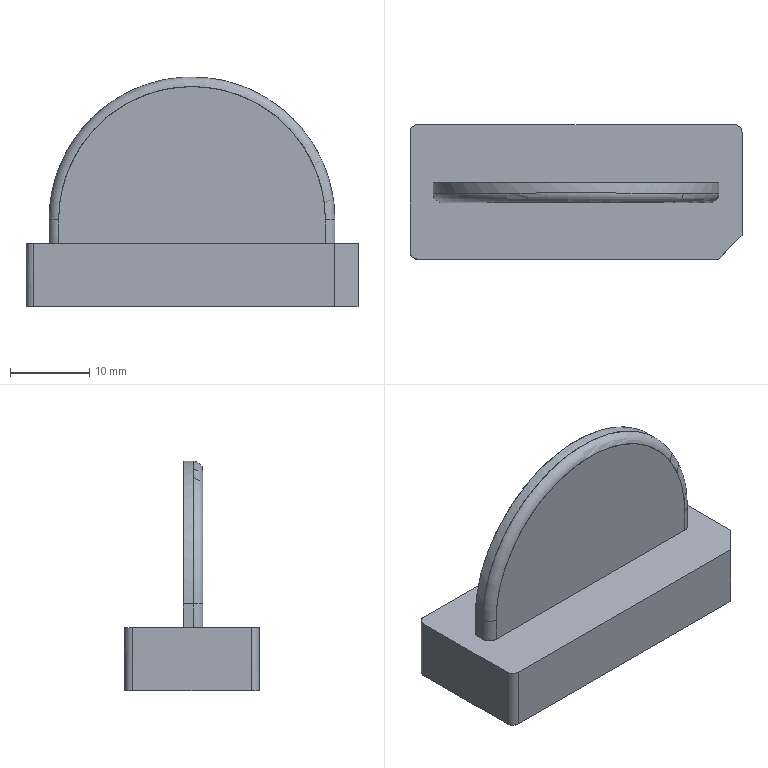NC program | PowerMill | posted with a generic post | part box 42 x 17 x 29.081 mm
Lines 14349 to 15047 of 145628:
N14446 M6
N14447 S18000 M03
N14448 G00 G90 X0.0 Y0.0
N14449 G43 Z10.798 H7
N14450
N14451 G05 P10000 R8
N14452 X19.2751 Y-2.1794
N14453 Z-19.2241
N14454 G01 Z-20.4241 F1200.0
N14455 X19.275 Y-2.1795 Z-20.2759 F2000.0
N14456 X19.2748 Y-2.1796 Z-20.2573
N14457 X19.2725 Y-2.1819 Z-20.1811
N14458 X19.2673 Y-2.1872 Z-20.0904
N14459 X19.2619 Y-2.1926 Z-20.0169
N14460 X19.2569 Y-2.1976 Z-19.9571
N14461 X19.2492 Y-2.2053 Z-19.8956
N14462 X19.2381 Y-2.2163 Z-19.8291
N14463 X19.2231 Y-2.2314 Z-19.7547
N14464 X19.2025 Y-2.252 Z-19.6656
N14465 X19.1985 Y-2.256 Z-19.6511
N14466 X19.1938 Y-2.2606 Z-19.637
N14467 X19.1865 Y-2.268 Z-19.6166
N14468 X19.1776 Y-2.2769 Z-19.5934
N14469 X19.1714 Y-2.2831 Z-19.5786
N14470 X19.1653 Y-2.2891 Z-19.5656
N14471 X19.1292 Y-2.3253 Z-19.5125
N14472 X19.0625 Y-2.392 Z-19.4813
N14473 X19.0133 Y-2.4412 Z-19.5198
N14474 X18.9993 Y-2.4552 Z-19.5402
N14475 X18.9861 Y-2.4683 Z-19.5629
N14476 X18.9759 Y-2.4786 Z-19.586
N14477 X18.9669 Y-2.4875 Z-19.6121
N14478 X18.959 Y-2.4955 Z-19.639
N14479 X18.9531 Y-2.5013 Z-19.6603
N14480 X18.9478 Y-2.5067 Z-19.6819
N14481 X18.9427 Y-2.5118 Z-19.7036
N14482 X18.9354 Y-2.5191 Z-19.7361
N14483 X18.9308 Y-2.5237 Z-19.758
N14484 X18.9266 Y-2.5279 Z-19.78
N14485 X18.9224 Y-2.5321 Z-19.8055
N14486 X18.9129 Y-2.5416 Z-19.8656
N14487 X18.9047 Y-2.5498 Z-19.9261
N14488 X18.8988 Y-2.5557 Z-19.9872
N14489 X18.8944 Y-2.5601 Z-20.0485
N14490 X18.8904 Y-2.5641 Z-20.1099
N14491 Z-20.1215
N14492 X18.8897 Y-2.5647 Z-20.2091
N14493 X18.8875 Y-2.567 Z-20.2763
N14494 X18.8874 Y-2.5671 Z-20.4235
N14495 X18.8013 Y-2.6369 Z-20.3989
N14496 X18.7127 Y-2.7036 Z-20.3742
N14497 X18.6217 Y-2.7671 Z-20.3496
N14498 X18.6066 Y-2.7772 Z-20.3456
N14499 Z-20.268
N14500 X18.6083 Y-2.7755 Z-20.1987
N14501 X18.6085 Y-2.7753 Z-20.1449
N14502 X18.6109 Y-2.7729 Z-20.0062
N14503 X18.6161 Y-2.7677 Z-19.8643
N14504 X18.6242 Y-2.7595 Z-19.7189
N14505 X18.6329 Y-2.7509 Z-19.6004
N14506 X18.6409 Y-2.7429 Z-19.5043
N14507 X18.65 Y-2.7337 Z-19.4084
N14508 X18.6613 Y-2.7224 Z-19.3129
N14509 X18.675 Y-2.7088 Z-19.2181
N14510 X18.69 Y-2.6937 Z-19.1236
N14511 X18.7028 Y-2.681 Z-19.0474
N14512 X18.7181 Y-2.6657 Z-18.9706
N14513 X18.7367 Y-2.647 Z-18.8916
N14514 X18.7587 Y-2.6251 Z-18.8107
N14515 X18.7831 Y-2.6007 Z-18.731
N14516 X18.7923 Y-2.5915 Z-18.7055
N14517 X18.8023 Y-2.5814 Z-18.6807
N14518 X18.817 Y-2.5668 Z-18.6469
N14519 X18.8281 Y-2.5557 Z-18.623
N14520 X18.8396 Y-2.5441 Z-18.5995
N14521 X18.852 Y-2.5318 Z-18.5768
N14522 X18.8729 Y-2.5109 Z-18.544
N14523 X18.8922 Y-2.4916 Z-18.5182
N14524 X18.911 Y-2.4728 Z-18.4977
N14525 X18.9297 Y-2.4541 Z-18.4817
N14526 X18.9473 Y-2.4365 Z-18.4705
N14527 X19.013 Y-2.3708 Z-18.4544
N14528 X19.088 Y-2.2957 Z-18.4839
N14529 X19.1086 Y-2.2752 Z-18.5007
N14530 X19.1295 Y-2.2543 Z-18.5222
N14531 X19.1514 Y-2.2324 Z-18.5494
N14532 X19.1702 Y-2.2135 Z-18.576
N14533 X19.1904 Y-2.1934 Z-18.6077
N14534 X19.2089 Y-2.1749 Z-18.6413
N14535 X19.2257 Y-2.158 Z-18.6767
N14536 X19.2483 Y-2.1355 Z-18.7258
N14537 X19.263 Y-2.1207 Z-18.7606
N14538 X19.2746 Y-2.1091 Z-18.7912
N14539 X19.2857 Y-2.0981 Z-18.8222
N14540 X19.2964 Y-2.0873 Z-18.8534
N14541 X19.3067 Y-2.0771 Z-18.885
N14542 X19.3277 Y-2.0561 Z-18.9543
N14543 X19.3469 Y-2.0369 Z-19.0247
N14544 X19.3642 Y-2.0196 Z-19.0963
N14545 X19.3796 Y-2.0041 Z-19.1685
N14546 X19.3937 Y-1.99 Z-19.2414
N14547 X19.4069 Y-1.9768 Z-19.3145
N14548 X19.4192 Y-1.9646 Z-19.3879
N14549 X19.4334 Y-1.9504 Z-19.4875
N14550 X19.447 Y-1.9368 Z-19.6012
N14551 X19.457 Y-1.9268 Z-19.6985
N14552 X19.4641 Y-1.9197 Z-19.7821
N14553 X19.4698 Y-1.914 Z-19.8659
N14554 X19.4745 Y-1.9093 Z-19.9499
N14555 X19.4783 Y-1.9055 Z-20.0339
N14556 X19.4809 Y-1.9029 Z-20.118
N14557 X19.4838 Y-1.9 Z-20.2678
N14558 X19.4839 Y-1.8999 Z-20.2719
N14559 Z-20.4005
N14560 X19.5967 Y-1.7163 Z-20.4082
N14561 Y-1.7164 Z-20.2636
N14562 X19.5954 Y-1.7176 Z-20.1838
N14563 X19.593 Y-1.72 Z-20.0648
N14564 X19.5895 Y-1.7235 Z-19.9459
N14565 X19.5843 Y-1.7287 Z-19.8271
N14566 X19.5771 Y-1.736 Z-19.7086
N14567 X19.5678 Y-1.7453 Z-19.5904
N14568 X19.5567 Y-1.7564 Z-19.4725
N14569 X19.5442 Y-1.7688 Z-19.3548
N14570 X19.5295 Y-1.7836 Z-19.2354
N14571 X19.5113 Y-1.8017 Z-19.1112
N14572 X19.4896 Y-1.8235 Z-18.9814
N14573 X19.4715 Y-1.8416 Z-18.8839
N14574 X19.4518 Y-1.8613 Z-18.787
N14575 X19.43 Y-1.8831 Z-18.691
N14576 X19.4059 Y-1.9072 Z-18.5961
N14577 X19.3798 Y-1.9333 Z-18.5023
N14578 X19.3617 Y-1.9513 Z-18.441
N14579 X19.3423 Y-1.9708 Z-18.3805
N14580 X19.3183 Y-1.9948 Z-18.3123
N14581 X19.2928 Y-2.0203 Z-18.246
N14582 X19.2687 Y-2.0444 Z-18.1891
N14583 X19.2472 Y-2.0659 Z-18.1428
N14584 X19.2172 Y-2.0959 Z-18.0828
N14585 X19.1911 Y-2.1219 Z-18.0354
N14586 X19.1652 Y-2.1479 Z-17.9941
N14587 X19.1386 Y-2.1745 Z-17.9572
N14588 X19.1112 Y-2.2018 Z-17.9245
N14589 X19.083 Y-2.23 Z-17.8958
N14590 X19.0593 Y-2.2538 Z-17.8752
N14591 X19.0331 Y-2.28 Z-17.8562
N14592 X19.0076 Y-2.3054 Z-17.8418
N14593 X18.933 Y-2.3801 Z-17.8264
N14594 X18.8661 Y-2.4469 Z-17.8455
N14595 X18.8556 Y-2.4574 Z-17.8528
N14596 X18.8354 Y-2.4776 Z-17.8676
N14597 X18.8157 Y-2.4974 Z-17.8837
N14598 X18.7969 Y-2.5162 Z-17.9018
N14599 X18.7795 Y-2.5336 Z-17.9224
N14600 X18.7634 Y-2.5497 Z-17.9452
N14601 X18.7483 Y-2.5647 Z-17.9694
N14602 X18.7339 Y-2.5792 Z-17.9943
N14603 X18.7197 Y-2.5933 Z-18.0196
N14604 X18.706 Y-2.6071 Z-18.0456
N14605 X18.686 Y-2.627 Z-18.0888
N14606 X18.666 Y-2.6471 Z-18.139
N14607 X18.6454 Y-2.6676 Z-18.198
N14608 X18.6241 Y-2.689 Z-18.2672
N14609 X18.6087 Y-2.7044 Z-18.3219
N14610 X18.5873 Y-2.7258 Z-18.406
N14611 X18.5667 Y-2.7464 Z-18.4977
N14612 X18.5469 Y-2.7662 Z-18.5978
N14613 X18.528 Y-2.7851 Z-18.7076
N14614 X18.5099 Y-2.8031 Z-18.8281
N14615 X18.4932 Y-2.8199 Z-18.9586
N14616 X18.4788 Y-2.8343 Z-19.089
N14617 X18.4675 Y-2.8456 Z-19.2077
N14618 X18.4566 Y-2.8565 Z-19.3393
N14619 X18.4452 Y-2.8679 Z-19.5083
N14620 X18.4361 Y-2.877 Z-19.6847
N14621 X18.4293 Y-2.8838 Z-19.8699
N14622 X18.4248 Y-2.8882 Z-20.0655
N14623 X18.4228 Y-2.8902 Z-20.2739
N14624 Y-2.8903 Z-20.3992
N14625 X18.2717 Y-2.9707 Z-20.3936
N14626 Y-2.9706 Z-20.2572
N14627 X18.2734 Y-2.969 Z-20.047
N14628 X18.2772 Y-2.9651 Z-19.8369
N14629 X18.2836 Y-2.9588 Z-19.6269
N14630 X18.2925 Y-2.9499 Z-19.417
N14631 X18.299 Y-2.9434 Z-19.2977
N14632 X18.3066 Y-2.9357 Z-19.1785
N14633 X18.3153 Y-2.927 Z-19.0594
N14634 X18.3251 Y-2.9173 Z-18.9406
N14635 X18.3359 Y-2.9064 Z-18.8219
N14636 X18.3482 Y-2.8941 Z-18.7035
N14637 X18.3625 Y-2.8799 Z-18.5855
N14638 X18.3824 Y-2.8599 Z-18.4374
N14639 X18.4025 Y-2.8398 Z-18.3062
N14640 X18.4233 Y-2.819 Z-18.1868
N14641 X18.4345 Y-2.8078 Z-18.1292
N14642 X18.4467 Y-2.7957 Z-18.0719
N14643 X18.4624 Y-2.78 Z-18.0041
N14644 X18.4833 Y-2.759 Z-17.9214
N14645 X18.5067 Y-2.7357 Z-17.8382
N14646 X18.5274 Y-2.7149 Z-17.7711
N14647 X18.5464 Y-2.696 Z-17.7154
N14648 X18.5662 Y-2.6761 Z-17.6628
N14649 X18.5829 Y-2.6594 Z-17.623
N14650 X18.6017 Y-2.6406 Z-17.5814
N14651 X18.6226 Y-2.6197 Z-17.54
N14652 X18.643 Y-2.5994 Z-17.5052
N14653 X18.662 Y-2.5804 Z-17.4769
N14654 X18.6811 Y-2.5612 Z-17.4504
N14655 X18.7008 Y-2.5415 Z-17.4255
N14656 X18.7217 Y-2.5207 Z-17.4022
N14657 X18.7442 Y-2.4981 Z-17.3813
N14658 X18.7671 Y-2.4753 Z-17.3646
N14659 X18.7901 Y-2.4523 Z-17.3515
N14660 X18.8135 Y-2.4288 Z-17.3411
N14661 X18.8268 Y-2.4155 Z-17.3362
N14662 X18.8988 Y-2.3435 Z-17.3319
N14663 X18.9749 Y-2.2674 Z-17.3595
N14664 X19.0036 Y-2.2388 Z-17.3791
N14665 X19.0314 Y-2.2109 Z-17.4009
N14666 X19.0588 Y-2.1835 Z-17.4254
N14667 X19.0861 Y-2.1562 Z-17.4538
N14668 X19.1137 Y-2.1286 Z-17.4871
N14669 X19.1409 Y-2.1014 Z-17.5248
N14670 X19.166 Y-2.0764 Z-17.5635
N14671 X19.1895 Y-2.0529 Z-17.6026
N14672 X19.2128 Y-2.0296 Z-17.6435
N14673 X19.2445 Y-1.9979 Z-17.7043
N14674 X19.2757 Y-1.9667 Z-17.7706
N14675 X19.3065 Y-1.9358 Z-17.8433
N14676 X19.3375 Y-1.9048 Z-17.9237
N14677 X19.3687 Y-1.8736 Z-18.0123
N14678 X19.4003 Y-1.842 Z-18.1104
N14679 X19.4308 Y-1.8116 Z-18.2144
N14680 X19.4602 Y-1.7821 Z-18.3252
N14681 X19.4889 Y-1.7535 Z-18.4439
N14682 X19.5161 Y-1.7263 Z-18.5683
N14683 X19.5413 Y-1.7011 Z-18.6967
N14684 X19.5647 Y-1.6776 Z-18.8308
N14685 X19.5839 Y-1.6585 Z-18.9546
N14686 X19.6047 Y-1.6377 Z-19.1055
N14687 X19.6141 Y-1.6282 Z-19.178
N14688 X19.6193 Y-1.623 Z-19.2232
N14689 X19.6241 Y-1.6183 Z-19.2684
N14690 X19.6287 Y-1.6137 Z-19.3138
N14691 X19.6346 Y-1.6077 Z-19.3748
N14692 X19.6389 Y-1.6034 Z-19.4202
N14693 X19.6431 Y-1.5992 Z-19.4656
N14694 X19.6472 Y-1.5952 Z-19.511
N14695 X19.6507 Y-1.5916 Z-19.5565
N14696 X19.6612 Y-1.5812 Z-19.7184
N14697 X19.669 Y-1.5733 Z-19.8806
N14698 X19.6743 Y-1.5681 Z-20.043
N14699 X19.677 Y-1.5654 Z-20.2055
N14700 X19.6774 Y-1.565 Z-20.2613
N14701 Y-1.5649 Z-20.4071
N14702 X19.7399 Y-1.4318 Z-20.3857
N14703 X19.7398 Z-20.2587
N14704 X19.7389 Y-1.4327 Z-20.1459
N14705 X19.7369 Y-1.4348 Z-20.0211
N14706 X19.7331 Y-1.4385 Z-19.8964
N14707 X19.7282 Y-1.4435 Z-19.7718
N14708 X19.7201 Y-1.4515 Z-19.6232
N14709 X19.7099 Y-1.4617 Z-19.4748
N14710 X19.6978 Y-1.4739 Z-19.3268
N14711 X19.6836 Y-1.488 Z-19.179
N14712 X19.6677 Y-1.5039 Z-19.0359
N14713 X19.6493 Y-1.5223 Z-18.8933
N14714 X19.6287 Y-1.543 Z-18.7514
N14715 X19.6059 Y-1.5658 Z-18.6101
N14716 X19.583 Y-1.5887 Z-18.4812
N14717 X19.5579 Y-1.6138 Z-18.3532
N14718 X19.5303 Y-1.6414 Z-18.2261
N14719 X19.5002 Y-1.6715 Z-18.1003
N14720 X19.4714 Y-1.7002 Z-17.989
N14721 X19.4401 Y-1.7316 Z-17.8782
N14722 X19.4053 Y-1.7664 Z-17.7659
N14723 X19.374 Y-1.7977 Z-17.672
N14724 X19.3413 Y-1.8303 Z-17.5811
N14725 X19.3098 Y-1.8619 Z-17.5008
N14726 X19.2776 Y-1.8941 Z-17.4261
N14727 X19.242 Y-1.9297 Z-17.3498
N14728 X19.2077 Y-1.964 Z-17.2826
N14729 X19.1739 Y-1.9978 Z-17.2224
N14730 X19.1397 Y-2.0319 Z-17.1675
N14731 X19.1071 Y-2.0645 Z-17.1194
N14732 X19.0783 Y-2.0934 Z-17.0811
N14733 X19.0504 Y-2.1212 Z-17.0488
N14734 X19.017 Y-2.1547 Z-17.0135
N14735 X18.9883 Y-2.1833 Z-16.9868
N14736 X18.9624 Y-2.2093 Z-16.9664
N14737 X18.9378 Y-2.2339 Z-16.9503
N14738 X18.9126 Y-2.2591 Z-16.936
N14739 X18.8864 Y-2.2853 Z-16.9245
N14740 X18.8599 Y-2.3118 Z-16.9167
N14741 X18.833 Y-2.3386 Z-16.912
N14742 X18.806 Y-2.3656 Z-16.9096
N14743 X18.7828 Y-2.3888 Z-16.9121
N14744 X18.7564 Y-2.4152 Z-16.9165
N14745 X18.7351 Y-2.4366 Z-16.923
N14746 X18.7129 Y-2.4587 Z-16.9326
N14747 X18.6899 Y-2.4818 Z-16.9454
N14748 X18.6662 Y-2.5055 Z-16.9621
N14749 X18.6425 Y-2.5291 Z-16.9824
N14750 X18.6215 Y-2.5501 Z-17.003
N14751 X18.602 Y-2.5696 Z-17.0242
N14752 X18.5833 Y-2.5884 Z-17.0484
N14753 X18.5625 Y-2.6091 Z-17.0791
N14754 X18.5391 Y-2.6325 Z-17.1184
N14755 X18.5123 Y-2.6593 Z-17.1688
N14756 X18.4912 Y-2.6805 Z-17.2125
N14757 X18.4751 Y-2.6965 Z-17.2483
N14758 X18.4624 Y-2.7092 Z-17.2784
N14759 X18.4504 Y-2.7212 Z-17.3089
N14760 X18.4364 Y-2.7352 Z-17.3472
N14761 X18.4134 Y-2.7582 Z-17.4162
N14762 X18.3907 Y-2.781 Z-17.4922
N14763 X18.3676 Y-2.804 Z-17.5781
N14764 X18.3443 Y-2.8274 Z-17.6755
N14765 X18.321 Y-2.8506 Z-17.784
N14766 X18.3013 Y-2.8704 Z-17.8874
N14767 X18.2855 Y-2.8862 Z-17.9787
N14768 X18.2725 Y-2.8991 Z-18.0604
N14769 X18.2511 Y-2.9206 Z-18.2108
N14770 X18.2321 Y-2.9395 Z-18.3635
N14771 X18.216 Y-2.9556 Z-18.5153
N14772 X18.1995 Y-2.9721 Z-18.6921
N14773 X18.1853 Y-2.9864 Z-18.8694
N14774 X18.1734 Y-2.9982 Z-19.047
N14775 X18.1614 Y-3.0103 Z-19.2724
N14776 X18.1518 Y-3.0198 Z-19.5036
N14777 X18.1448 Y-3.0269 Z-19.7415
N14778 X18.1403 Y-3.0314 Z-19.9866
N14779 X18.1384 Y-3.0332 Z-20.2398
N14780 Z-20.3023
N14781 X18.0175 Y-3.0834 Z-20.2284
N14782 X18.0187 Y-3.0823 Z-20.0336
N14783 X18.0208 Y-3.0801 Z-19.8389
N14784 X18.0257 Y-3.0752 Z-19.5953
N14785 X18.0332 Y-3.0678 Z-19.3519
N14786 X18.0432 Y-3.0577 Z-19.1086
N14787 X18.0494 Y-3.0515 Z-18.9806
N14788 X18.0565 Y-3.0444 Z-18.8526
N14789 X18.0646 Y-3.0363 Z-18.7247
N14790 X18.0746 Y-3.0263 Z-18.5847
N14791 X18.0881 Y-3.0128 Z-18.4189
N14792 X18.1051 Y-2.9958 Z-18.2376
N14793 X18.1214 Y-2.9795 Z-18.0854
N14794 X18.1372 Y-2.9637 Z-17.9548
N14795 X18.1543 Y-2.9466 Z-17.8288
N14796 X18.1734 Y-2.9275 Z-17.7034
N14797 X18.1895 Y-2.9115 Z-17.609
N14798 X18.212 Y-2.8889 Z-17.4869
N14799 X18.2337 Y-2.8672 Z-17.382
N14800 X18.2557 Y-2.8453 Z-17.2883
N14801 X18.2795 Y-2.8214 Z-17.197
N14802 X18.3047 Y-2.7963 Z-17.1091
N14803 X18.3294 Y-2.7715 Z-17.0317
N14804 X18.3543 Y-2.7466 Z-16.9623
N14805 X18.3797 Y-2.7212 Z-16.8994
N14806 X18.4059 Y-2.695 Z-16.8419
N14807 X18.433 Y-2.668 Z-16.7893
N14808 X18.4611 Y-2.6398 Z-16.7411
N14809 X18.4904 Y-2.6106 Z-16.6968
N14810 X18.5161 Y-2.5848 Z-16.6627
N14811 X18.5425 Y-2.5584 Z-16.6327
N14812 X18.5695 Y-2.5314 Z-16.6068
N14813 X18.597 Y-2.5039 Z-16.5851
N14814 X18.625 Y-2.4759 Z-16.5674
N14815 X18.6533 Y-2.4476 Z-16.5537
N14816 X18.682 Y-2.4189 Z-16.5439
N14817 X18.7109 Y-2.39 Z-16.5381
N14818 X18.7401 Y-2.3609 Z-16.5362
N14819 X18.7694 Y-2.3315 Z-16.538
N14820 X18.7989 Y-2.3021 Z-16.5437
N14821 X18.8285 Y-2.2724 Z-16.5532
N14822 X18.8604 Y-2.2406 Z-16.5673
N14823 X18.8926 Y-2.2083 Z-16.5856
N14824 X18.9253 Y-2.1757 Z-16.6084
N14825 X18.9582 Y-2.1427 Z-16.6357
N14826 X18.9913 Y-2.1096 Z-16.6676
N14827 X19.0241 Y-2.0768 Z-16.7038
N14828 X19.056 Y-2.0449 Z-16.7437
N14829 X19.0798 Y-2.0211 Z-16.776
N14830 X19.109 Y-1.9919 Z-16.8171
N14831 X19.1372 Y-1.9637 Z-16.8594
N14832 X19.1638 Y-1.9371 Z-16.9038
N14833 X19.1889 Y-1.9121 Z-16.95
N14834 X19.2129 Y-1.888 Z-16.9974
N14835 X19.2365 Y-1.8645 Z-17.0451
N14836 X19.2597 Y-1.8412 Z-17.0931
N14837 X19.2925 Y-1.8084 Z-17.1653
N14838 X19.3234 Y-1.7775 Z-17.2391
N14839 X19.3553 Y-1.7456 Z-17.3223
N14840 X19.3825 Y-1.7184 Z-17.3991
N14841 X19.4086 Y-1.6924 Z-17.4767
N14842 X19.4337 Y-1.6672 Z-17.5547
N14843 X19.4639 Y-1.637 Z-17.6537
N14844 X19.4922 Y-1.6087 Z-17.7539
N14845 X19.5185 Y-1.5824 Z-17.8551
N14846 X19.5432 Y-1.5577 Z-17.9572
N14847 X19.5669 Y-1.5341 Z-18.0598
N14848 X19.5941 Y-1.5068 Z-18.1871
N14849 X19.6192 Y-1.4817 Z-18.3154
N14850 X19.6446 Y-1.4564 Z-18.4575
N14851 X19.6667 Y-1.4342 Z-18.594
N14852 X19.6858 Y-1.4151 Z-18.7243
N14853 X19.703 Y-1.3979 Z-18.8552
N14854 X19.7232 Y-1.3777 Z-19.0275
N14855 X19.7411 Y-1.3599 Z-19.2025
N14856 X19.7552 Y-1.3458 Z-19.3651
N14857 X19.7667 Y-1.3343 Z-19.5282
N14858 X19.7765 Y-1.3244 Z-19.7077
N14859 X19.7838 Y-1.3171 Z-19.8906
N14860 X19.7884 Y-1.3125 Z-20.0771
N14861 X19.7902 Y-1.3107 Z-20.2642
N14862 X19.7903 Y-1.3106 Z-20.3894
N14863 X19.8316 Y-1.1986 Z-20.3952
N14864 X19.8315 Y-1.1987 Z-20.2317
N14865 X19.8305 Y-1.1997 Z-20.1264
N14866 X19.8273 Y-1.2029 Z-19.9514
N14867 X19.8218 Y-1.2084 Z-19.7764
N14868 X19.8138 Y-1.2165 Z-19.6006
N14869 X19.8032 Y-1.227 Z-19.4261
N14870 X19.7902 Y-1.24 Z-19.252
N14871 X19.7773 Y-1.2529 Z-19.1042
N14872 X19.7624 Y-1.2678 Z-18.9568
N14873 X19.7456 Y-1.2846 Z-18.8098
N14874 X19.7244 Y-1.3058 Z-18.6448
N14875 X19.7036 Y-1.3266 Z-18.4989
N14876 X19.6806 Y-1.3496 Z-18.3536
N14877 X19.6573 Y-1.3729 Z-18.22
N14878 X19.6324 Y-1.3978 Z-18.087
N14879 X19.6057 Y-1.4246 Z-17.9548
N14880 X19.5761 Y-1.4542 Z-17.8206
N14881 X19.5448 Y-1.4855 Z-17.6904
N14882 X19.5112 Y-1.519 Z-17.5614
N14883 X19.4817 Y-1.5485 Z-17.4554
N14884 X19.4452 Y-1.5851 Z-17.3326
N14885 X19.408 Y-1.6222 Z-17.2175
N14886 X19.3702 Y-1.6601 Z-17.109
N14887 X19.3314 Y-1.6988 Z-17.0065
N14888 X19.2911 Y-1.7391 Z-16.9081
N14889 X19.2511 Y-1.7791 Z-16.8176
N14890 X19.2117 Y-1.8185 Z-16.7352
N14891 X19.1725 Y-1.8577 Z-16.6596
N14892 X19.1487 Y-1.8815 Z-16.617
N14893 X19.1158 Y-1.9144 Z-16.5619
N14894 X19.0774 Y-1.9528 Z-16.5023
N14895 X19.0449 Y-1.9853 Z-16.4557
N14896 X19.0167 Y-2.0135 Z-16.4185
N14897 X18.9881 Y-2.0421 Z-16.3842
N14898 X18.965 Y-2.0652 Z-16.3592
N14899 X18.9266 Y-2.1036 Z-16.3207
N14900 X18.8912 Y-2.139 Z-16.2891
N14901 X18.8577 Y-2.1725 Z-16.2632
N14902 X18.8255 Y-2.2047 Z-16.2424
N14903 X18.794 Y-2.2363 Z-16.2261
N14904 X18.7628 Y-2.2674 Z-16.2139
N14905 X18.7317 Y-2.2985 Z-16.2055
N14906 X18.7005 Y-2.3297 Z-16.2008
N14907 X18.669 Y-2.3612 Z-16.1996
N14908 X18.6401 Y-2.3901 Z-16.2014
N14909 X18.6111 Y-2.4191 Z-16.207
N14910 X18.5822 Y-2.448 Z-16.2164
N14911 X18.5533 Y-2.4769 Z-16.2299
N14912 X18.5243 Y-2.5059 Z-16.2475
N14913 X18.4954 Y-2.5348 Z-16.2694
N14914 X18.4666 Y-2.5636 Z-16.2956
N14915 X18.4381 Y-2.5922 Z-16.3263
N14916 X18.4098 Y-2.6204 Z-16.3615
N14917 X18.3823 Y-2.6479 Z-16.4011
N14918 X18.3557 Y-2.6745 Z-16.4447
N14919 X18.3286 Y-2.7017 Z-16.4953
N14920 X18.3018 Y-2.7284 Z-16.5512
N14921 X18.2753 Y-2.7549 Z-16.6132
N14922 X18.2491 Y-2.7811 Z-16.6817
N14923 X18.2231 Y-2.8071 Z-16.7576
N14924 X18.1973 Y-2.833 Z-16.8416
N14925 X18.1718 Y-2.8584 Z-16.934
N14926 X18.1473 Y-2.8829 Z-17.0334
N14927 X18.1259 Y-2.9044 Z-17.1296
N14928 X18.1081 Y-2.9221 Z-17.217
N14929 X18.0965 Y-2.9337 Z-17.2786
N14930 X18.0784 Y-2.9518 Z-17.384
N14931 X18.0618 Y-2.9684 Z-17.4899
N14932 X18.0452 Y-2.985 Z-17.6051
N14933 X18.031 Y-2.9992 Z-17.7118
N14934 X18.018 Y-3.0122 Z-17.8187
N14935 X18.0006 Y-3.0296 Z-17.9818
N14936 X17.9841 Y-3.0462 Z-18.159
N14937 X17.9685 Y-3.0618 Z-18.3523
N14938 X17.9537 Y-3.0766 Z-18.5687
N14939 X17.941 Y-3.0892 Z-18.79
N14940 X17.9316 Y-3.0986 Z-18.9875
N14941 X17.9244 Y-3.1058 Z-19.166
N14942 X17.9164 Y-3.1138 Z-19.4193
N14943 X17.9107 Y-3.1195 Z-19.6727
N14944 X17.9071 Y-3.1232 Z-19.9262
N14945 X17.9055 Y-3.1247 Z-20.1797
N14946 X17.8 Y-3.1595 Z-20.1798
N14947 X17.8002 Y-3.1593 Z-20.0866
N14948 X17.8028 Y-3.1567 Z-19.8064
N14949 X17.8071 Y-3.1524 Z-19.5262
N14950 X17.8123 Y-3.1472 Z-19.3008
N14951 X17.821 Y-3.1385 Z-19.0149
N14952 X17.8316 Y-3.1279 Z-18.7491
N14953 X17.8442 Y-3.1153 Z-18.4989
N14954 X17.8588 Y-3.1007 Z-18.2615
N14955 X17.8753 Y-3.0842 Z-18.0347
N14956 X17.8854 Y-3.0741 Z-17.9136
N14957 X17.8972 Y-3.0623 Z-17.7843
N14958 X17.9121 Y-3.0474 Z-17.6387
N14959 X17.9309 Y-3.0287 Z-17.4764
N14960 X17.9517 Y-3.0078 Z-17.3178
N14961 X17.9727 Y-2.9868 Z-17.1757
N14962 X17.9939 Y-2.9656 Z-17.0486
N14963 X18.0153 Y-2.9442 Z-16.9327
N14964 X18.039 Y-2.9205 Z-16.8177
N14965 X18.0559 Y-2.9036 Z-16.7435
N14966 X18.0763 Y-2.8832 Z-16.6614
N14967 X18.101 Y-2.8585 Z-16.5711
N14968 X18.1278 Y-2.8318 Z-16.4831
N14969 X18.1544 Y-2.8051 Z-16.404
N14970 X18.1807 Y-2.7788 Z-16.334
N14971 X18.2066 Y-2.7529 Z-16.2719
N14972 X18.2322 Y-2.7273 Z-16.2169
N14973 X18.2581 Y-2.7014 Z-16.1671
N14974 X18.2864 Y-2.6731 Z-16.1183
N14975 X18.3148 Y-2.6447 Z-16.0753
N14976 X18.3432 Y-2.6163 Z-16.0374
N14977 X18.3718 Y-2.5877 Z-16.0043
N14978 X18.4006 Y-2.5589 Z-15.9757
N14979 X18.4298 Y-2.5297 Z-15.9514
N14980 X18.4593 Y-2.5002 Z-15.9313
N14981 X18.4893 Y-2.4702 Z-15.9151
N14982 X18.5196 Y-2.4399 Z-15.9027
N14983 X18.5505 Y-2.409 Z-15.8941
N14984 X18.5817 Y-2.3778 Z-15.8892
N14985 X18.6134 Y-2.3461 Z-15.8878
N14986 X18.6452 Y-2.3144 Z-15.89
N14987 X18.677 Y-2.2825 Z-15.8958
N14988 X18.7091 Y-2.2505 Z-15.9054
N14989 X18.7417 Y-2.2178 Z-15.9192
N14990 X18.7752 Y-2.1843 Z-15.9374
N14991 X18.8102 Y-2.1493 Z-15.9605
N14992 X18.8472 Y-2.1123 Z-15.9891
N14993 X18.8851 Y-2.0744 Z-16.022
N14994 X18.9152 Y-2.0443 Z-16.0515
N14995 X18.9444 Y-2.0152 Z-16.0835
N14996 X18.9774 Y-1.9821 Z-16.1235
N14997 X19.0157 Y-1.9438 Z-16.1741
N14998 X19.054 Y-1.9055 Z-16.2292
N14999 X19.0842 Y-1.8753 Z-16.2756
N15000 X19.1083 Y-1.8512 Z-16.3149
N15001 X19.1315 Y-1.828 Z-16.355
N15002 X19.1742 Y-1.7853 Z-16.4335
N15003 X19.2162 Y-1.7433 Z-16.5172
N15004 X19.2576 Y-1.7019 Z-16.6064
N15005 X19.2986 Y-1.6609 Z-16.7019
N15006 X19.3394 Y-1.6201 Z-16.8044
N15007 X19.3802 Y-1.5793 Z-16.915
N15008 X19.4206 Y-1.5389 Z-17.0326
N15009 X19.4593 Y-1.5002 Z-17.1544
N15010 X19.4963 Y-1.4632 Z-17.2805
N15011 X19.5347 Y-1.4248 Z-17.421
N15012 X19.5713 Y-1.3882 Z-17.566
N15013 X19.6061 Y-1.3534 Z-17.7161
N15014 X19.6393 Y-1.3202 Z-17.8715
N15015 X19.6708 Y-1.2887 Z-18.0326
N15016 X19.6966 Y-1.2629 Z-18.1773
N15017 X19.7213 Y-1.2382 Z-18.3293
N15018 X19.7451 Y-1.2144 Z-18.4913
N15019 X19.7667 Y-1.1928 Z-18.6534
N15020 X19.7852 Y-1.1743 Z-18.8071
N15021 X19.8018 Y-1.1578 Z-18.9613
N15022 X19.8165 Y-1.143 Z-19.12
N15023 X19.8294 Y-1.1301 Z-19.279
N15024 X19.8404 Y-1.1191 Z-19.4383
N15025 X19.8494 Y-1.1102 Z-19.5979
N15026 X19.8568 Y-1.1027 Z-19.7703
N15027 X19.8619 Y-1.0976 Z-19.943
N15028 X19.8649 Y-1.0946 Z-20.1158
N15029 X19.8661 Y-1.0934 Z-20.2607
N15030 X19.8662 Y-1.0933 Z-20.4013
N15031 X19.8952 Y-0.9936 Z-20.4072
N15032 X19.8951 Y-0.9937 Z-20.2396
N15033 X19.8948 Y-0.994 Z-20.1765
N15034 X19.8919 Y-0.9969 Z-19.9727
N15035 X19.8864 Y-1.0024 Z-19.7717
N15036 X19.8781 Y-1.0107 Z-19.5737
N15037 X19.8672 Y-1.0216 Z-19.3784
N15038 X19.8536 Y-1.0352 Z-19.1858
N15039 X19.8374 Y-1.0514 Z-18.9955
N15040 X19.8184 Y-1.0704 Z-18.8043
N15041 X19.7973 Y-1.0915 Z-18.6197
N15042 X19.7739 Y-1.1149 Z-18.4389
N15043 X19.7475 Y-1.1413 Z-18.2563
N15044 X19.7191 Y-1.1697 Z-18.0794
N15045 X19.6889 Y-1.1999 Z-17.9078
N15046 X19.6566 Y-1.2322 Z-17.7412
N15047 X19.6246 Y-1.2642 Z-17.5892
N15048 X19.5897 Y-1.2991 Z-17.4372
N15049 X19.5528 Y-1.3359 Z-17.2894
N15050 X19.5139 Y-1.3749 Z-17.1445
N15051 X19.474 Y-1.4148 Z-17.0064
N15052 X19.4339 Y-1.4549 Z-16.8772
N15053 X19.3934 Y-1.4954 Z-16.7557
N15054 X19.3522 Y-1.5366 Z-16.6409
N15055 X19.3101 Y-1.5787 Z-16.5319
N15056 X19.266 Y-1.6228 Z-16.4257
N15057 X19.2247 Y-1.6641 Z-16.3329
N15058 X19.1822 Y-1.7066 Z-16.244
N15059 X19.1394 Y-1.7494 Z-16.1608
N15060 X19.0968 Y-1.792 Z-16.0841
N15061 X19.0544 Y-1.8344 Z-16.0139
N15062 X19.0123 Y-1.8765 Z-15.9498
N15063 X18.9705 Y-1.9183 Z-15.8916
N15064 X18.9289 Y-1.9599 Z-15.8388
N15065 X18.8874 Y-2.0014 Z-15.7912
N15066 X18.8495 Y-2.0393 Z-15.7519
N15067 X18.8114 Y-2.0774 Z-15.7169
N15068 X18.7735 Y-2.1153 Z-15.6864
N15069 X18.736 Y-2.1528 Z-15.6606
N15070 X18.6991 Y-2.1897 Z-15.6394
N15071 X18.6629 Y-2.2259 Z-15.6226
N15072 X18.6274 Y-2.2614 Z-15.6101
N15073 X18.5942 Y-2.2946 Z-15.602
N15074 X18.5614 Y-2.3274 Z-15.5977
N15075 X18.5288 Y-2.36 Z-15.5971
N15076 X18.4965 Y-2.3923 Z-15.6003
N15077 X18.4646 Y-2.4242 Z-15.6073
N15078 X18.433 Y-2.4558 Z-15.6182
N15079 X18.4017 Y-2.487 Z-15.6331
N15080 X18.3709 Y-2.5179 Z-15.652
N15081 X18.3404 Y-2.5484 Z-15.6749
N15082 X18.3102 Y-2.5786 Z-15.702
N15083 X18.2806 Y-2.6082 Z-15.7334
N15084 X18.2513 Y-2.6375 Z-15.7691
N15085 X18.2225 Y-2.6663 Z-15.8092
N15086 X18.2021 Y-2.6867 Z-15.8409
N15087 X18.173 Y-2.7158 Z-15.8908
N15088 X18.1445 Y-2.7443 Z-15.9458
N15089 X18.1164 Y-2.7724 Z-16.0062
N15090 X18.0889 Y-2.7999 Z-16.0726
N15091 X18.0617 Y-2.8271 Z-16.1454
N15092 X18.035 Y-2.8538 Z-16.2253
N15093 X18.0088 Y-2.88 Z-16.3128
N15094 X17.9832 Y-2.9056 Z-16.4079
N15095 X17.9588 Y-2.93 Z-16.5089
N15096 X17.9374 Y-2.9514 Z-16.607
N15097 X17.9194 Y-2.9693 Z-16.6969
N15098 X17.9045 Y-2.9843 Z-16.7778
N15099 X17.8932 Y-2.9956 Z-16.8426
N15100 X17.872 Y-3.0168 Z-16.9756
N15101 X17.8519 Y-3.0369 Z-17.117
N15102 X17.8312 Y-3.0576 Z-17.2805
N15103 X17.8143 Y-3.0745 Z-17.4319
N15104 X17.8008 Y-3.088 Z-17.5669
N15105 X17.7865 Y-3.1023 Z-17.7274
N15106 X17.7717 Y-3.1171 Z-17.9187
N15107 X17.7588 Y-3.13 Z-18.1103
N15108 X17.7464 Y-3.1424 Z-18.3237
N15109 X17.7346 Y-3.1542 Z-18.5658
N15110 X17.7266 Y-3.1622 Z-18.7608
N15111 X17.7199 Y-3.1689 Z-18.9531
N15112 X17.7144 Y-3.1744 Z-19.1455
N15113 X17.7075 Y-3.1813 Z-19.4591
N15114 X17.7027 Y-3.1861 Z-19.7924
N15115 X17.7003 Y-3.1885 Z-20.1258
N15116 X17.7002 Y-3.1886 Z-20.1832
N15117 X17.6051 Y-3.213 Z-20.1897
N15118 X17.6052 Y-3.2129 Z-20.1488
N15119 X17.6065 Y-3.2116 Z-19.8823
N15120 X17.6091 Y-3.209 Z-19.6158
N15121 X17.613 Y-3.2051 Z-19.3493
N15122 X17.6184 Y-3.1997 Z-19.0829
N15123 X17.6255 Y-3.1925 Z-18.8166
N15124 X17.6334 Y-3.1847 Z-18.5865
N15125 X17.6426 Y-3.1755 Z-18.3565
N15126 X17.6537 Y-3.1644 Z-18.1267
N15127 X17.6669 Y-3.1512 Z-17.8972
N15128 X17.6745 Y-3.1436 Z-17.7777
N15129 X17.6831 Y-3.1349 Z-17.6583
N15130 X17.6926 Y-3.1255 Z-17.5391
N15131 X17.7026 Y-3.1155 Z-17.42
N15132 X17.7133 Y-3.1047 Z-17.301
N15133 X17.7241 Y-3.094 Z-17.1919
N15134 X17.7363 Y-3.0818 Z-17.0822
N15135 X17.7513 Y-3.0668 Z-16.9585
N15136 X17.77 Y-3.0481 Z-16.8187
N15137 X17.7924 Y-3.0257 Z-16.6688
N15138 X17.8152 Y-3.0029 Z-16.5333
N15139 X17.8378 Y-2.9803 Z-16.4129
N15140 X17.8602 Y-2.9579 Z-16.3053
N15141 X17.8833 Y-2.9348 Z-16.2053
N15142 X17.9034 Y-2.9147 Z-16.1264
N15143 X17.9283 Y-2.8898 Z-16.0373
N15144 X17.9553 Y-2.8628 Z-15.9506